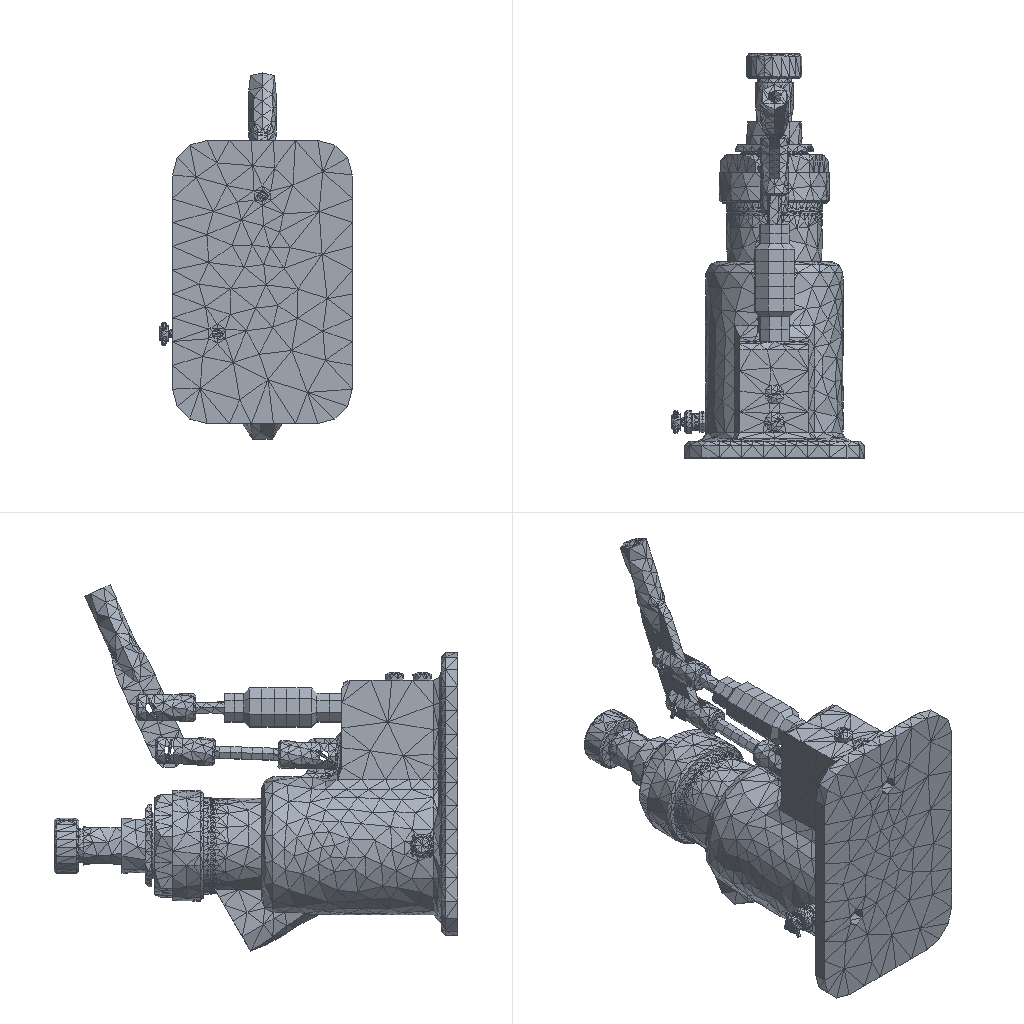Simulation study | ansys workbench
Set-up summary:
category,name,step,type,value,unit,region
solver,ansys_workbench
units,mm-N-s-tonne (MPa),,stated,"/units,MPA"
analysis,deck-1/LS1,,static
load_step,deck-1/LS1,deck-1/LS1,static,nsubst=1; time=1
analysis,deck-2/LS1,,modal,method=lanb; n_modes=30
load_step,deck-2/LS1,deck-2/LS1,modal
mesh,deck-1.dat,,nodes,324920
mesh,deck-1.dat,,elements,213612
element_type,SOLID187,,,178759,,deck-1.dat
element_type,TARGE170,,,16183,,deck-1.dat
element_type,CONTA174,,,16183,,deck-1.dat
element_type,SOLID186,,,1800,,deck-1.dat
element_type,SURF154,,,687,,deck-1.dat
mesh,deck-2.dat,,nodes,58677
mesh,deck-2.dat,,elements,39683
element_type,SOLID187,,,29823,,deck-2.dat
element_type,TARGE170,,,4803,,deck-2.dat
element_type,CONTA174,,,4803,,deck-2.dat
element_type,SOLID186,,,254,,deck-2.dat
material,Structural Steel,,E,200000,tonne s^-2 mm^-1
material,Structural Steel,,nu,0.3
material,Structural Steel,,density,7.85e-09,tonne mm^-3
material,Structural Steel,,conductivity,60.5,tonne mm s^-3 C^-1
material,Structural Steel,,specific_heat,4.34e+08,mm^2 s^-2 C^-1
material,Structural Steel,,cte,1.2e-05,C^-1
material,Structural Steel,,permeability,10000
material,Structural Steel,,resistivity,0.00017,ohm mm
material,Structural Steel,,E,200000,tonne s^-2 mm^-1
material,Structural Steel,,nu,0.3
material,Structural Steel,,density,7.85e-09,tonne mm^-3
material,Structural Steel,,conductivity,60.5,tonne mm s^-3 C^-1
material,Structural Steel,,specific_heat,4.34e+08,mm^2 s^-2 C^-1
material,Structural Steel,,cte,1.2e-05,C^-1
material,Structural Steel,,permeability,10000
material,Structural Steel,,resistivity,0.00017,ohm mm
load,Define Force Using Surface Effect Elements,deck-1/LS1,surface-effect pres face 2,-1.14,,SURF154 #78
bc,Fixed Supports,deck-1/model,fixed,[dofs=ALL],,_FIXEDSU
contact,Contact Region,,bonded (always),element=CONTA174
contact,Contact Region 2,,bonded (always),element=CONTA174
contact,Contact Region 3,,bonded (always),element=CONTA174
contact,Contact Region 4,,bonded (always),element=CONTA174
contact,Contact Region 5,,bonded (always),element=CONTA174
contact,Contact Region 6,,bonded (always),element=CONTA174
contact,Contact Region 7,,bonded (always),element=CONTA174
contact,Contact Region 8,,bonded (always),element=CONTA174
contact,Contact Region 9,,bonded (always),element=CONTA174
contact,Contact Region 10,,bonded (always),element=CONTA174
contact,Contact Region 11,,bonded (always),element=CONTA174
contact,Contact Region 12,,bonded (always),element=CONTA174
contact,Contact Region 13,,bonded (always),element=CONTA174
contact,Contact Region 14,,bonded (always),element=CONTA174
contact,Contact Region 15,,bonded (always),element=CONTA174
contact,Contact Region 16,,bonded (always),element=CONTA174
contact,Contact Region 17,,bonded (always),element=CONTA174
contact,Contact Region 18,,bonded (always),element=CONTA174
contact,Contact Region 19,,bonded (always),element=CONTA174
contact,Contact Region 20,,bonded (always),element=CONTA174
contact,Contact Region 21,,bonded (always),element=CONTA174
contact,Contact Region 22,,bonded (always),element=CONTA174
contact,Contact Region 24,,bonded (always),element=CONTA174
contact,Contact Region 25,,bonded (always),element=CONTA174
contact,Contact Region 26,,bonded (always),element=CONTA174
contact,Contact Region 27,,bonded (always),element=CONTA174
contact,Contact Region 29,,bonded (always),element=CONTA174
contact,Contact Region,,bonded (always),element=CONTA174
contact,Contact Region 2,,bonded (always),element=CONTA174
contact,Contact Region 3,,bonded (always),element=CONTA174
contact,Contact Region 4,,bonded (always),element=CONTA174
contact,Contact Region 5,,bonded (always),element=CONTA174
contact,Contact Region 6,,bonded (always),element=CONTA174
contact,Contact Region 7,,bonded (always),element=CONTA174
contact,Contact Region 8,,bonded (always),element=CONTA174
contact,Contact Region 9,,bonded (always),element=CONTA174
contact,Contact Region 10,,bonded (always),element=CONTA174
contact,Contact Region 11,,bonded (always),element=CONTA174
contact,Contact Region 12,,bonded (always),element=CONTA174
contact,Contact Region 13,,bonded (always),element=CONTA174
contact,Contact Region 14,,bonded (always),element=CONTA174
contact,Contact Region 15,,bonded (always),element=CONTA174
contact,Contact Region 16,,bonded (always),element=CONTA174
contact,Contact Region 17,,bonded (always),element=CONTA174
contact,Contact Region 18,,bonded (always),element=CONTA174
contact,Contact Region 19,,bonded (always),element=CONTA174
contact,Contact Region 20,,bonded (always),element=CONTA174
contact,Contact Region 21,,bonded (always),element=CONTA174
contact,Contact Region 22,,bonded (always),element=CONTA174
contact,Contact Region 23,,bonded (always),element=CONTA174
contact,Contact Region 24,,bonded (always),element=CONTA174
contact,Contact Region 25,,bonded (always),element=CONTA174
contact,Contact Region 26,,bonded (always),element=CONTA174
contact,Contact Region 27,,bonded (always),element=CONTA174
contact,Contact Region 28,,bonded (always),element=CONTA174
contact,Contact Region 29,,bonded (always),element=CONTA174
named_set,_FIXEDSU,,node,16408
Results summary:
result,analyses[0].index,,,1
result,analyses[0].system,,,SYS
result,analyses[0].deck,,,deck-1.dat
result,analyses[0].solve_status,,,completed
result,analyses[0].analysis_type,,,static
result,analyses[0].physics,,,mechanical
result,analyses[0].unit_system,,,"NMM: mm, ton, N, s, mV, mA, degC"
result,analyses[0].n_sets,,,1
result,analyses[0].load_steps[0].set,set=1,,1
result,analyses[0].load_steps[0].time_or_freq,set=1,,1
result,analyses[0].load_steps[0].max_displacement_magnitude,set=1,,0.02559
result,analyses[0].load_steps[0].max_von_mises_nodal,set=1,,161.446
result,analyses[0].load_steps[0].reaction_force_sum_xyz[1],set=1,,1.18312e-05
result,analyses[0].load_steps[0].reaction_force_sum_xyz[2],set=1,,4999.99
result,analyses[0].load_steps[0].reaction_force_sum_xyz[3],set=1,,1.79487e-05
result,analyses[1].index,,,2
result,analyses[1].system,,,SYS-1
result,analyses[1].deck,,,deck-2.dat
result,analyses[1].solve_status,,,completed
result,analyses[1].analysis_type,,,modal
result,analyses[1].physics,,,mechanical
result,analyses[1].unit_system,,,"NMM: mm, ton, N, s, mV, mA, degC"
result,analyses[1].n_sets,,,30
result,analyses[1].modal_frequencies_hz[1],,,0
result,analyses[1].modal_frequencies_hz[2],,,0
result,analyses[1].modal_frequencies_hz[3],,,0
result,analyses[1].modal_frequencies_hz[4],,,0
result,analyses[1].modal_frequencies_hz[5],,,0
result,analyses[1].modal_frequencies_hz[6],,,0
result,analyses[1].modal_frequencies_hz[7],,,0
result,analyses[1].modal_frequencies_hz[8],,,0
result,analyses[1].modal_frequencies_hz[9],,,0
result,analyses[1].modal_frequencies_hz[10],,,0
result,analyses[1].modal_frequencies_hz[11],,,0
result,analyses[1].modal_frequencies_hz[12],,,0
result,analyses[1].modal_frequencies_hz[13],,,0
result,analyses[1].modal_frequencies_hz[14],,,0
result,analyses[1].modal_frequencies_hz[15],,,0
result,analyses[1].modal_frequencies_hz[16],,,0
result,analyses[1].modal_frequencies_hz[17],,,0.0004852
result,analyses[1].modal_frequencies_hz[18],,,0.002866
result,analyses[1].modal_frequencies_hz[19],,,0.005318
result,analyses[1].modal_frequencies_hz[20],,,0.006877
result,analyses[1].modal_frequencies_hz[21],,,0.01005
result,analyses[1].modal_frequencies_hz[22],,,0.01021
result,analyses[1].modal_frequencies_hz[23],,,0.01072
result,analyses[1].modal_frequencies_hz[24],,,0.01308
result,analyses[1].modal_frequencies_hz[25],,,0.01424
result,analyses[1].modal_frequencies_hz[26],,,0.01431
result,analyses[1].modal_frequencies_hz[27],,,0.01539
result,analyses[1].modal_frequencies_hz[28],,,0.01613
result,analyses[1].modal_frequencies_hz[29],,,0.01705
result,analyses[1].modal_frequencies_hz[30],,,0.01816